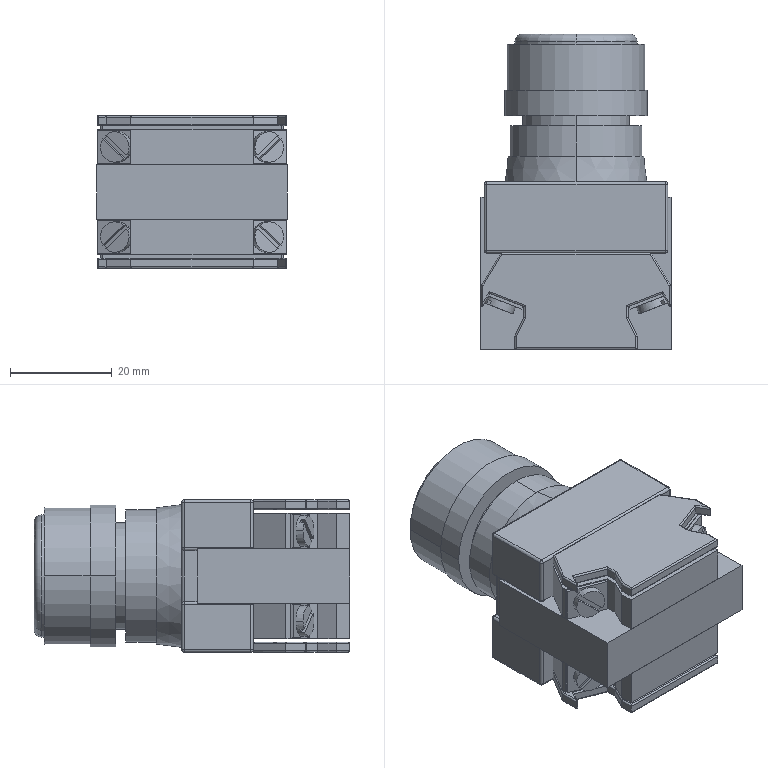Part | SolidWorks | features BaseBody 3, Fillet 1, ICE 1 | 3 solids | 280 faces | box 37.364 x 62 x 30 mm | volume 48495 mm3 | plane 132 | cylinder 120 | spline 24 | torus 2 | cone 2 | commonest cylinder face diameters 0.6 x64 1 x34 6 x8 0.24 x4 21 x2 24 x2